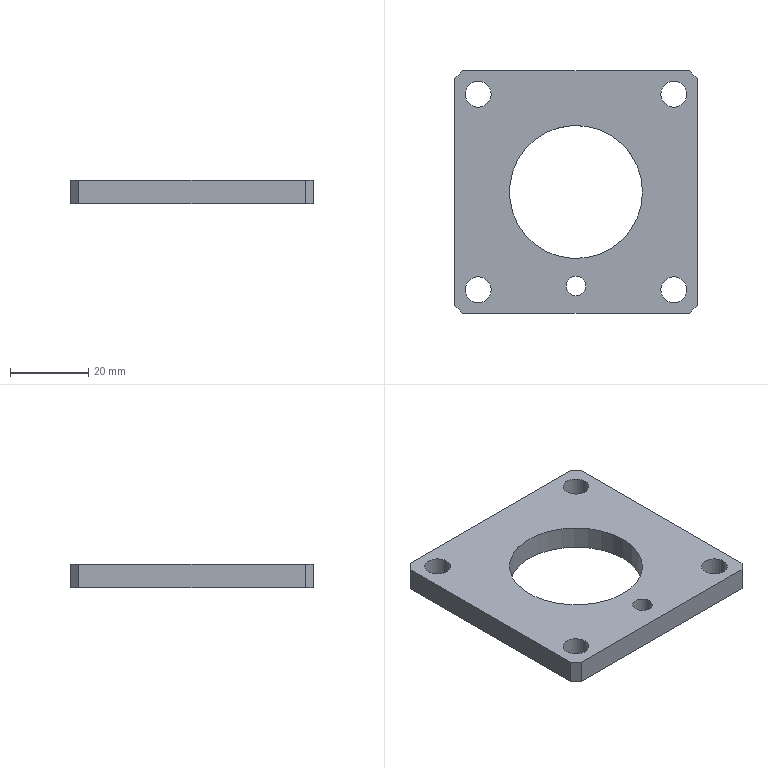Part | NX | features EXTRUDE 2, DATUM_CSYS 1 | 1 solid | 16 faces | box 62 x 62 x 6 mm | volume 16618 mm3 | plane 10 | cylinder 6 | commonest cylinder face diameters 6.647 x4 5 x1 34 x1
STEP:
#1=CARTESIAN_POINT('',(4156.983,6895.83,-25.133));
#2=VERTEX_POINT('',#1);
#3=CARTESIAN_POINT('',(4153.659,6895.83,-25.133));
#4=DIRECTION('',(0.,0.,1.));
#5=DIRECTION('',(1.,0.,0.));
#6=AXIS2_PLACEMENT_3D('',#3,#4,#5);
#7=CIRCLE('',#6,3.324);
#8=EDGE_CURVE('',#2,#2,#7,.T.);
#9=ORIENTED_EDGE('',*,*,#8,.T.);
#10=EDGE_LOOP('',(#9));
#11=FACE_BOUND('',#10,.T.);
#12=CARTESIAN_POINT('',(4131.159,6896.83,-25.133));
#13=VERTEX_POINT('',#12);
#14=CARTESIAN_POINT('',(4128.659,6896.83,-25.133));
#15=DIRECTION('',(0.,0.,1.));
#16=DIRECTION('',(1.,0.,0.));
#17=AXIS2_PLACEMENT_3D('',#14,#15,#16);
#18=CIRCLE('',#17,2.5);
#19=EDGE_CURVE('',#13,#13,#18,.T.);
#20=ORIENTED_EDGE('',*,*,#19,.T.);
#21=EDGE_LOOP('',(#20));
#22=FACE_BOUND('',#21,.T.);
#23=CARTESIAN_POINT('',(4145.659,6920.83,-25.133));
#24=VERTEX_POINT('',#23);
#25=CARTESIAN_POINT('',(4128.659,6920.83,-25.133));
#26=DIRECTION('',(0.,0.,1.));
#27=DIRECTION('',(1.,0.,0.));
#28=AXIS2_PLACEMENT_3D('',#25,#26,#27);
#29=CIRCLE('',#28,17.);
#30=EDGE_CURVE('',#24,#24,#29,.T.);
#31=ORIENTED_EDGE('',*,*,#30,.T.);
#32=EDGE_LOOP('',(#31));
#33=FACE_BOUND('',#32,.T.);
#34=CARTESIAN_POINT('',(4106.983,6895.83,-25.133));
#35=VERTEX_POINT('',#34);
#36=CARTESIAN_POINT('',(4103.659,6895.83,-25.133));
#37=DIRECTION('',(0.,0.,1.));
#38=DIRECTION('',(1.,0.,0.));
#39=AXIS2_PLACEMENT_3D('',#36,#37,#38);
#40=CIRCLE('',#39,3.324);
#41=EDGE_CURVE('',#35,#35,#40,.T.);
#42=ORIENTED_EDGE('',*,*,#41,.T.);
#43=EDGE_LOOP('',(#42));
#44=FACE_BOUND('',#43,.T.);
#45=CARTESIAN_POINT('',(4156.983,6945.83,-25.133));
#46=VERTEX_POINT('',#45);
#47=CARTESIAN_POINT('',(4153.659,6945.83,-25.133));
#48=DIRECTION('',(0.,0.,1.));
#49=DIRECTION('',(1.,0.,0.));
#50=AXIS2_PLACEMENT_3D('',#47,#48,#49);
#51=CIRCLE('',#50,3.324);
#52=EDGE_CURVE('',#46,#46,#51,.T.);
#53=ORIENTED_EDGE('',*,*,#52,.T.);
#54=EDGE_LOOP('',(#53));
#55=FACE_BOUND('',#54,.T.);
#56=CARTESIAN_POINT('',(4157.659,6951.83,-25.133));
#57=VERTEX_POINT('',#56);
#58=CARTESIAN_POINT('',(4099.659,6951.83,-25.133));
#59=VERTEX_POINT('',#58);
#60=CARTESIAN_POINT('',(4157.659,6951.83,-25.133));
#61=DIRECTION('',(-1.,0.,0.));
#62=VECTOR('',#61,1000.);
#63=LINE('',#60,#62);
#64=EDGE_CURVE('',#57,#59,#63,.T.);
#65=ORIENTED_EDGE('',*,*,#64,.F.);
#66=CARTESIAN_POINT('',(4159.659,6949.83,-25.133));
#67=VERTEX_POINT('',#66);
#68=CARTESIAN_POINT('',(4159.659,6949.83,-25.133));
#69=DIRECTION('',(-0.7071,0.7071,0.));
#70=VECTOR('',#69,1000.);
#71=LINE('',#68,#70);
#72=EDGE_CURVE('',#67,#57,#71,.T.);
#73=ORIENTED_EDGE('',*,*,#72,.F.);
#74=CARTESIAN_POINT('',(4159.659,6891.83,-25.133));
#75=VERTEX_POINT('',#74);
#76=CARTESIAN_POINT('',(4159.659,6891.83,-25.133));
#77=DIRECTION('',(0.,1.,0.));
#78=VECTOR('',#77,1000.);
#79=LINE('',#76,#78);
#80=EDGE_CURVE('',#75,#67,#79,.T.);
#81=ORIENTED_EDGE('',*,*,#80,.F.);
#82=CARTESIAN_POINT('',(4157.659,6889.83,-25.133));
#83=VERTEX_POINT('',#82);
#84=CARTESIAN_POINT('',(4157.659,6889.83,-25.133));
#85=DIRECTION('',(0.7071,0.7071,0.));
#86=VECTOR('',#85,1000.);
#87=LINE('',#84,#86);
#88=EDGE_CURVE('',#83,#75,#87,.T.);
#89=ORIENTED_EDGE('',*,*,#88,.F.);
#90=CARTESIAN_POINT('',(4099.659,6889.83,-25.133));
#91=VERTEX_POINT('',#90);
#92=CARTESIAN_POINT('',(4099.659,6889.83,-25.133));
#93=DIRECTION('',(1.,0.,0.));
#94=VECTOR('',#93,1000.);
#95=LINE('',#92,#94);
#96=EDGE_CURVE('',#91,#83,#95,.T.);
#97=ORIENTED_EDGE('',*,*,#96,.F.);
#98=CARTESIAN_POINT('',(4097.659,6891.83,-25.133));
#99=VERTEX_POINT('',#98);
#100=CARTESIAN_POINT('',(4097.659,6891.83,-25.133));
#101=DIRECTION('',(0.7071,-0.7071,0.));
#102=VECTOR('',#101,1000.);
#103=LINE('',#100,#102);
#104=EDGE_CURVE('',#99,#91,#103,.T.);
#105=ORIENTED_EDGE('',*,*,#104,.F.);
#106=CARTESIAN_POINT('',(4097.659,6949.83,-25.133));
#107=VERTEX_POINT('',#106);
#108=CARTESIAN_POINT('',(4097.659,6949.83,-25.133));
#109=DIRECTION('',(0.,-1.,0.));
#110=VECTOR('',#109,1000.);
#111=LINE('',#108,#110);
#112=EDGE_CURVE('',#107,#99,#111,.T.);
#113=ORIENTED_EDGE('',*,*,#112,.F.);
#114=CARTESIAN_POINT('',(4099.659,6951.83,-25.133));
#115=DIRECTION('',(-0.7071,-0.7071,0.));
#116=VECTOR('',#115,1000.);
#117=LINE('',#114,#116);
#118=EDGE_CURVE('',#59,#107,#117,.T.);
#119=ORIENTED_EDGE('',*,*,#118,.F.);
#120=EDGE_LOOP('',(#65,#73,#81,#89,#97,#105,#113,#119));
#121=FACE_BOUND('',#120,.T.);
#122=CARTESIAN_POINT('',(4106.983,6945.83,-25.133));
#123=VERTEX_POINT('',#122);
#124=CARTESIAN_POINT('',(4103.659,6945.83,-25.133));
#125=DIRECTION('',(0.,0.,-1.));
#126=DIRECTION('',(1.,0.,0.));
#127=AXIS2_PLACEMENT_3D('',#124,#125,#126);
#128=CIRCLE('',#127,3.324);
#129=EDGE_CURVE('',#123,#123,#128,.T.);
#130=ORIENTED_EDGE('',*,*,#129,.F.);
#131=EDGE_LOOP('',(#130));
#132=FACE_BOUND('',#131,.T.);
#133=CARTESIAN_POINT('',(0.,0.,-25.133));
#134=DIRECTION('',(0.,0.,1.));
#135=DIRECTION('',(0.,-1.,0.));
#136=AXIS2_PLACEMENT_3D('',#133,#134,#135);
#137=PLANE('',#136);
#138=ADVANCED_FACE('',(#11,#22,#33,#44,#55,#121,#132),#137,.F.);
#139=CARTESIAN_POINT('',(4157.659,6951.83,-19.133));
#140=VERTEX_POINT('',#139);
#141=CARTESIAN_POINT('',(4099.659,6951.83,-19.133));
#142=VERTEX_POINT('',#141);
#143=CARTESIAN_POINT('',(4157.659,6951.83,-19.133));
#144=DIRECTION('',(-1.,0.,0.));
#145=VECTOR('',#144,1000.);
#146=LINE('',#143,#145);
#147=EDGE_CURVE('',#140,#142,#146,.T.);
#148=ORIENTED_EDGE('',*,*,#147,.T.);
#149=CARTESIAN_POINT('',(4097.659,6949.83,-19.133));
#150=VERTEX_POINT('',#149);
#151=CARTESIAN_POINT('',(4099.659,6951.83,-19.133));
#152=DIRECTION('',(-0.7071,-0.7071,0.));
#153=VECTOR('',#152,1000.);
#154=LINE('',#151,#153);
#155=EDGE_CURVE('',#142,#150,#154,.T.);
#156=ORIENTED_EDGE('',*,*,#155,.T.);
#157=CARTESIAN_POINT('',(4097.659,6891.83,-19.133));
#158=VERTEX_POINT('',#157);
#159=CARTESIAN_POINT('',(4097.659,6949.83,-19.133));
#160=DIRECTION('',(0.,-1.,0.));
#161=VECTOR('',#160,1000.);
#162=LINE('',#159,#161);
#163=EDGE_CURVE('',#150,#158,#162,.T.);
#164=ORIENTED_EDGE('',*,*,#163,.T.);
#165=CARTESIAN_POINT('',(4099.659,6889.83,-19.133));
#166=VERTEX_POINT('',#165);
#167=CARTESIAN_POINT('',(4097.659,6891.83,-19.133));
#168=DIRECTION('',(0.7071,-0.7071,0.));
#169=VECTOR('',#168,1000.);
#170=LINE('',#167,#169);
#171=EDGE_CURVE('',#158,#166,#170,.T.);
#172=ORIENTED_EDGE('',*,*,#171,.T.);
#173=CARTESIAN_POINT('',(4157.659,6889.83,-19.133));
#174=VERTEX_POINT('',#173);
#175=CARTESIAN_POINT('',(4099.659,6889.83,-19.133));
#176=DIRECTION('',(1.,0.,0.));
#177=VECTOR('',#176,1000.);
#178=LINE('',#175,#177);
#179=EDGE_CURVE('',#166,#174,#178,.T.);
#180=ORIENTED_EDGE('',*,*,#179,.T.);
#181=CARTESIAN_POINT('',(4159.659,6891.83,-19.133));
#182=VERTEX_POINT('',#181);
#183=CARTESIAN_POINT('',(4157.659,6889.83,-19.133));
#184=DIRECTION('',(0.7071,0.7071,0.));
#185=VECTOR('',#184,1000.);
#186=LINE('',#183,#185);
#187=EDGE_CURVE('',#174,#182,#186,.T.);
#188=ORIENTED_EDGE('',*,*,#187,.T.);
#189=CARTESIAN_POINT('',(4159.659,6949.83,-19.133));
#190=VERTEX_POINT('',#189);
#191=CARTESIAN_POINT('',(4159.659,6891.83,-19.133));
#192=DIRECTION('',(0.,1.,0.));
#193=VECTOR('',#192,1000.);
#194=LINE('',#191,#193);
#195=EDGE_CURVE('',#182,#190,#194,.T.);
#196=ORIENTED_EDGE('',*,*,#195,.T.);
#197=CARTESIAN_POINT('',(4159.659,6949.83,-19.133));
#198=DIRECTION('',(-0.7071,0.7071,0.));
#199=VECTOR('',#198,1000.);
#200=LINE('',#197,#199);
#201=EDGE_CURVE('',#190,#140,#200,.T.);
#202=ORIENTED_EDGE('',*,*,#201,.T.);
#203=EDGE_LOOP('',(#148,#156,#164,#172,#180,#188,#196,#202));
#204=FACE_BOUND('',#203,.T.);
#205=CARTESIAN_POINT('',(4156.983,6945.83,-19.133));
#206=VERTEX_POINT('',#205);
#207=CARTESIAN_POINT('',(4153.659,6945.83,-19.133));
#208=DIRECTION('',(0.,0.,1.));
#209=DIRECTION('',(1.,0.,0.));
#210=AXIS2_PLACEMENT_3D('',#207,#208,#209);
#211=CIRCLE('',#210,3.324);
#212=EDGE_CURVE('',#206,#206,#211,.T.);
#213=ORIENTED_EDGE('',*,*,#212,.F.);
#214=EDGE_LOOP('',(#213));
#215=FACE_BOUND('',#214,.T.);
#216=CARTESIAN_POINT('',(4106.983,6895.83,-19.133));
#217=VERTEX_POINT('',#216);
#218=CARTESIAN_POINT('',(4103.659,6895.83,-19.133));
#219=DIRECTION('',(0.,0.,1.));
#220=DIRECTION('',(1.,0.,0.));
#221=AXIS2_PLACEMENT_3D('',#218,#219,#220);
#222=CIRCLE('',#221,3.324);
#223=EDGE_CURVE('',#217,#217,#222,.T.);
#224=ORIENTED_EDGE('',*,*,#223,.F.);
#225=EDGE_LOOP('',(#224));
#226=FACE_BOUND('',#225,.T.);
#227=CARTESIAN_POINT('',(4145.659,6920.83,-19.133));
#228=VERTEX_POINT('',#227);
#229=CARTESIAN_POINT('',(4128.659,6920.83,-19.133));
#230=DIRECTION('',(0.,0.,1.));
#231=DIRECTION('',(1.,0.,0.));
#232=AXIS2_PLACEMENT_3D('',#229,#230,#231);
#233=CIRCLE('',#232,17.);
#234=EDGE_CURVE('',#228,#228,#233,.T.);
#235=ORIENTED_EDGE('',*,*,#234,.F.);
#236=EDGE_LOOP('',(#235));
#237=FACE_BOUND('',#236,.T.);
#238=CARTESIAN_POINT('',(4131.159,6896.83,-19.133));
#239=VERTEX_POINT('',#238);
#240=CARTESIAN_POINT('',(4128.659,6896.83,-19.133));
#241=DIRECTION('',(0.,0.,1.));
#242=DIRECTION('',(1.,0.,0.));
#243=AXIS2_PLACEMENT_3D('',#240,#241,#242);
#244=CIRCLE('',#243,2.5);
#245=EDGE_CURVE('',#239,#239,#244,.T.);
#246=ORIENTED_EDGE('',*,*,#245,.F.);
#247=EDGE_LOOP('',(#246));
#248=FACE_BOUND('',#247,.T.);
#249=CARTESIAN_POINT('',(4156.983,6895.83,-19.133));
#250=VERTEX_POINT('',#249);
#251=CARTESIAN_POINT('',(4153.659,6895.83,-19.133));
#252=DIRECTION('',(0.,0.,1.));
#253=DIRECTION('',(1.,0.,0.));
#254=AXIS2_PLACEMENT_3D('',#251,#252,#253);
#255=CIRCLE('',#254,3.324);
#256=EDGE_CURVE('',#250,#250,#255,.T.);
#257=ORIENTED_EDGE('',*,*,#256,.F.);
#258=EDGE_LOOP('',(#257));
#259=FACE_BOUND('',#258,.T.);
#260=CARTESIAN_POINT('',(4106.983,6945.83,-19.133));
#261=VERTEX_POINT('',#260);
#262=CARTESIAN_POINT('',(4103.659,6945.83,-19.133));
#263=DIRECTION('',(0.,0.,-1.));
#264=DIRECTION('',(1.,0.,0.));
#265=AXIS2_PLACEMENT_3D('',#262,#263,#264);
#266=CIRCLE('',#265,3.324);
#267=EDGE_CURVE('',#261,#261,#266,.T.);
#268=ORIENTED_EDGE('',*,*,#267,.T.);
#269=EDGE_LOOP('',(#268));
#270=FACE_BOUND('',#269,.T.);
#271=CARTESIAN_POINT('',(0.,0.,-19.133));
#272=DIRECTION('',(0.,0.,1.));
#273=DIRECTION('',(0.,-1.,0.));
#274=AXIS2_PLACEMENT_3D('',#271,#272,#273);
#275=PLANE('',#274);
#276=ADVANCED_FACE('',(#204,#215,#226,#237,#248,#259,#270),#275,.T.);
#277=ORIENTED_EDGE('',*,*,#147,.F.);
#278=CARTESIAN_POINT('',(4157.659,6951.83,-25.133));
#279=DIRECTION('',(0.,0.,1.));
#280=VECTOR('',#279,1000.);
#281=LINE('',#278,#280);
#282=EDGE_CURVE('',#57,#140,#281,.T.);
#283=ORIENTED_EDGE('',*,*,#282,.F.);
#284=ORIENTED_EDGE('',*,*,#64,.T.);
#285=CARTESIAN_POINT('',(4099.659,6951.83,-25.133));
#286=DIRECTION('',(0.,0.,1.));
#287=VECTOR('',#286,1000.);
#288=LINE('',#285,#287);
#289=EDGE_CURVE('',#59,#142,#288,.T.);
#290=ORIENTED_EDGE('',*,*,#289,.T.);
#291=EDGE_LOOP('',(#277,#283,#284,#290));
#292=FACE_BOUND('',#291,.T.);
#293=CARTESIAN_POINT('',(4157.659,6951.83,-25.133));
#294=DIRECTION('',(0.,1.,0.));
#295=DIRECTION('',(0.,0.,1.));
#296=AXIS2_PLACEMENT_3D('',#293,#294,#295);
#297=PLANE('',#296);
#298=ADVANCED_FACE('',(#292),#297,.T.);
#299=ORIENTED_EDGE('',*,*,#155,.F.);
#300=ORIENTED_EDGE('',*,*,#289,.F.);
#301=ORIENTED_EDGE('',*,*,#118,.T.);
#302=CARTESIAN_POINT('',(4097.659,6949.83,-25.133));
#303=DIRECTION('',(0.,0.,1.));
#304=VECTOR('',#303,1000.);
#305=LINE('',#302,#304);
#306=EDGE_CURVE('',#107,#150,#305,.T.);
#307=ORIENTED_EDGE('',*,*,#306,.T.);
#308=EDGE_LOOP('',(#299,#300,#301,#307));
#309=FACE_BOUND('',#308,.T.);
#310=CARTESIAN_POINT('',(4099.659,6951.83,-25.133));
#311=DIRECTION('',(-0.7071,0.7071,0.));
#312=DIRECTION('',(-0.7071,-0.7071,0.));
#313=AXIS2_PLACEMENT_3D('',#310,#311,#312);
#314=PLANE('',#313);
#315=ADVANCED_FACE('',(#309),#314,.T.);
#316=ORIENTED_EDGE('',*,*,#163,.F.);
#317=ORIENTED_EDGE('',*,*,#306,.F.);
#318=ORIENTED_EDGE('',*,*,#112,.T.);
#319=CARTESIAN_POINT('',(4097.659,6891.83,-25.133));
#320=DIRECTION('',(0.,0.,1.));
#321=VECTOR('',#320,1000.);
#322=LINE('',#319,#321);
#323=EDGE_CURVE('',#99,#158,#322,.T.);
#324=ORIENTED_EDGE('',*,*,#323,.T.);
#325=EDGE_LOOP('',(#316,#317,#318,#324));
#326=FACE_BOUND('',#325,.T.);
#327=CARTESIAN_POINT('',(4097.659,6949.83,-25.133));
#328=DIRECTION('',(-1.,0.,0.));
#329=DIRECTION('',(0.,0.,1.));
#330=AXIS2_PLACEMENT_3D('',#327,#328,#329);
#331=PLANE('',#330);
#332=ADVANCED_FACE('',(#326),#331,.T.);
#333=ORIENTED_EDGE('',*,*,#171,.F.);
#334=ORIENTED_EDGE('',*,*,#323,.F.);
#335=ORIENTED_EDGE('',*,*,#104,.T.);
#336=CARTESIAN_POINT('',(4099.659,6889.83,-25.133));
#337=DIRECTION('',(0.,0.,1.));
#338=VECTOR('',#337,1000.);
#339=LINE('',#336,#338);
#340=EDGE_CURVE('',#91,#166,#339,.T.);
#341=ORIENTED_EDGE('',*,*,#340,.T.);
#342=EDGE_LOOP('',(#333,#334,#335,#341));
#343=FACE_BOUND('',#342,.T.);
#344=CARTESIAN_POINT('',(4097.659,6891.83,-25.133));
#345=DIRECTION('',(-0.7071,-0.7071,0.));
#346=DIRECTION('',(0.7071,-0.7071,0.));
#347=AXIS2_PLACEMENT_3D('',#344,#345,#346);
#348=PLANE('',#347);
#349=ADVANCED_FACE('',(#343),#348,.T.);
#350=ORIENTED_EDGE('',*,*,#179,.F.);
#351=ORIENTED_EDGE('',*,*,#340,.F.);
#352=ORIENTED_EDGE('',*,*,#96,.T.);
#353=CARTESIAN_POINT('',(4157.659,6889.83,-25.133));
#354=DIRECTION('',(0.,0.,1.));
#355=VECTOR('',#354,1000.);
#356=LINE('',#353,#355);
#357=EDGE_CURVE('',#83,#174,#356,.T.);
#358=ORIENTED_EDGE('',*,*,#357,.T.);
#359=EDGE_LOOP('',(#350,#351,#352,#358));
#360=FACE_BOUND('',#359,.T.);
#361=CARTESIAN_POINT('',(4099.659,6889.83,-25.133));
#362=DIRECTION('',(0.,-1.,0.));
#363=DIRECTION('',(0.,0.,-1.));
#364=AXIS2_PLACEMENT_3D('',#361,#362,#363);
#365=PLANE('',#364);
#366=ADVANCED_FACE('',(#360),#365,.T.);
#367=ORIENTED_EDGE('',*,*,#187,.F.);
#368=ORIENTED_EDGE('',*,*,#357,.F.);
#369=ORIENTED_EDGE('',*,*,#88,.T.);
#370=CARTESIAN_POINT('',(4159.659,6891.83,-25.133));
#371=DIRECTION('',(0.,0.,1.));
#372=VECTOR('',#371,1000.);
#373=LINE('',#370,#372);
#374=EDGE_CURVE('',#75,#182,#373,.T.);
#375=ORIENTED_EDGE('',*,*,#374,.T.);
#376=EDGE_LOOP('',(#367,#368,#369,#375));
#377=FACE_BOUND('',#376,.T.);
#378=CARTESIAN_POINT('',(4157.659,6889.83,-25.133));
#379=DIRECTION('',(0.7071,-0.7071,0.));
#380=DIRECTION('',(0.7071,0.7071,0.));
#381=AXIS2_PLACEMENT_3D('',#378,#379,#380);
#382=PLANE('',#381);
#383=ADVANCED_FACE('',(#377),#382,.T.);
#384=ORIENTED_EDGE('',*,*,#195,.F.);
#385=ORIENTED_EDGE('',*,*,#374,.F.);
#386=ORIENTED_EDGE('',*,*,#80,.T.);
#387=CARTESIAN_POINT('',(4159.659,6949.83,-25.133));
#388=DIRECTION('',(0.,0.,1.));
#389=VECTOR('',#388,1000.);
#390=LINE('',#387,#389);
#391=EDGE_CURVE('',#67,#190,#390,.T.);
#392=ORIENTED_EDGE('',*,*,#391,.T.);
#393=EDGE_LOOP('',(#384,#385,#386,#392));
#394=FACE_BOUND('',#393,.T.);
#395=CARTESIAN_POINT('',(4159.659,6891.83,-25.133));
#396=DIRECTION('',(1.,0.,0.));
#397=DIRECTION('',(0.,0.,-1.));
#398=AXIS2_PLACEMENT_3D('',#395,#396,#397);
#399=PLANE('',#398);
#400=ADVANCED_FACE('',(#394),#399,.T.);
#401=ORIENTED_EDGE('',*,*,#201,.F.);
#402=ORIENTED_EDGE('',*,*,#391,.F.);
#403=ORIENTED_EDGE('',*,*,#72,.T.);
#404=ORIENTED_EDGE('',*,*,#282,.T.);
#405=EDGE_LOOP('',(#401,#402,#403,#404));
#406=FACE_BOUND('',#405,.T.);
#407=CARTESIAN_POINT('',(4159.659,6949.83,-25.133));
#408=DIRECTION('',(0.7071,0.7071,0.));
#409=DIRECTION('',(-0.7071,0.7071,0.));
#410=AXIS2_PLACEMENT_3D('',#407,#408,#409);
#411=PLANE('',#410);
#412=ADVANCED_FACE('',(#406),#411,.T.);
#413=ORIENTED_EDGE('',*,*,#52,.F.);
#414=EDGE_LOOP('',(#413));
#415=FACE_BOUND('',#414,.T.);
#416=ORIENTED_EDGE('',*,*,#212,.T.);
#417=EDGE_LOOP('',(#416));
#418=FACE_BOUND('',#417,.T.);
#419=CARTESIAN_POINT('',(4153.659,6945.83,-25.133));
#420=DIRECTION('',(0.,0.,1.));
#421=DIRECTION('',(1.,0.,0.));
#422=AXIS2_PLACEMENT_3D('',#419,#420,#421);
#423=CYLINDRICAL_SURFACE('',#422,3.324);
#424=ADVANCED_FACE('',(#415,#418),#423,.F.);
#425=ORIENTED_EDGE('',*,*,#41,.F.);
#426=EDGE_LOOP('',(#425));
#427=FACE_BOUND('',#426,.T.);
#428=ORIENTED_EDGE('',*,*,#223,.T.);
#429=EDGE_LOOP('',(#428));
#430=FACE_BOUND('',#429,.T.);
#431=CARTESIAN_POINT('',(4103.659,6895.83,-25.133));
#432=DIRECTION('',(0.,0.,1.));
#433=DIRECTION('',(1.,0.,0.));
#434=AXIS2_PLACEMENT_3D('',#431,#432,#433);
#435=CYLINDRICAL_SURFACE('',#434,3.324);
#436=ADVANCED_FACE('',(#427,#430),#435,.F.);
#437=ORIENTED_EDGE('',*,*,#30,.F.);
#438=EDGE_LOOP('',(#437));
#439=FACE_BOUND('',#438,.T.);
#440=ORIENTED_EDGE('',*,*,#234,.T.);
#441=EDGE_LOOP('',(#440));
#442=FACE_BOUND('',#441,.T.);
#443=CARTESIAN_POINT('',(4128.659,6920.83,-25.133));
#444=DIRECTION('',(0.,0.,1.));
#445=DIRECTION('',(1.,0.,0.));
#446=AXIS2_PLACEMENT_3D('',#443,#444,#445);
#447=CYLINDRICAL_SURFACE('',#446,17.);
#448=ADVANCED_FACE('',(#439,#442),#447,.F.);
#449=ORIENTED_EDGE('',*,*,#19,.F.);
#450=EDGE_LOOP('',(#449));
#451=FACE_BOUND('',#450,.T.);
#452=ORIENTED_EDGE('',*,*,#245,.T.);
#453=EDGE_LOOP('',(#452));
#454=FACE_BOUND('',#453,.T.);
#455=CARTESIAN_POINT('',(4128.659,6896.83,-25.133));
#456=DIRECTION('',(0.,0.,1.));
#457=DIRECTION('',(1.,0.,0.));
#458=AXIS2_PLACEMENT_3D('',#455,#456,#457);
#459=CYLINDRICAL_SURFACE('',#458,2.5);
#460=ADVANCED_FACE('',(#451,#454),#459,.F.);
#461=ORIENTED_EDGE('',*,*,#8,.F.);
#462=EDGE_LOOP('',(#461));
#463=FACE_BOUND('',#462,.T.);
#464=ORIENTED_EDGE('',*,*,#256,.T.);
#465=EDGE_LOOP('',(#464));
#466=FACE_BOUND('',#465,.T.);
#467=CARTESIAN_POINT('',(4153.659,6895.83,-25.133));
#468=DIRECTION('',(0.,0.,1.));
#469=DIRECTION('',(1.,0.,0.));
#470=AXIS2_PLACEMENT_3D('',#467,#468,#469);
#471=CYLINDRICAL_SURFACE('',#470,3.324);
#472=ADVANCED_FACE('',(#463,#466),#471,.F.);
#473=ORIENTED_EDGE('',*,*,#129,.T.);
#474=EDGE_LOOP('',(#473));
#475=FACE_BOUND('',#474,.T.);
#476=ORIENTED_EDGE('',*,*,#267,.F.);
#477=EDGE_LOOP('',(#476));
#478=FACE_BOUND('',#477,.T.);
#479=CARTESIAN_POINT('',(4103.659,6945.83,-25.133));
#480=DIRECTION('',(0.,0.,1.));
#481=DIRECTION('',(1.,0.,0.));
#482=AXIS2_PLACEMENT_3D('',#479,#480,#481);
#483=CYLINDRICAL_SURFACE('',#482,3.324);
#484=ADVANCED_FACE('',(#475,#478),#483,.F.);
#485=CLOSED_SHELL('',(#138,#276,#298,#315,#332,#349,#366,#383,#400,#412,#424,#436,#448,#460,#472,#484));
#486=MANIFOLD_SOLID_BREP('',#485);
#487=(LENGTH_UNIT()NAMED_UNIT(*)SI_UNIT(.MILLI.,.METRE.));
#488=UNCERTAINTY_MEASURE_WITH_UNIT(LENGTH_MEASURE(0.00001),#487,'','');
#489=(NAMED_UNIT(*)PLANE_ANGLE_UNIT()SI_UNIT($,.RADIAN.));
#490=(NAMED_UNIT(*)SI_UNIT($,.STERADIAN.)SOLID_ANGLE_UNIT());
#491=(GEOMETRIC_REPRESENTATION_CONTEXT(3)GLOBAL_UNCERTAINTY_ASSIGNED_CONTEXT((#488))GLOBAL_UNIT_ASSIGNED_CONTEXT((#487,#489,#490))REPRESENTATION_CONTEXT('',''));
#492=ADVANCED_BREP_SHAPE_REPRESENTATION('',(#486),#491);